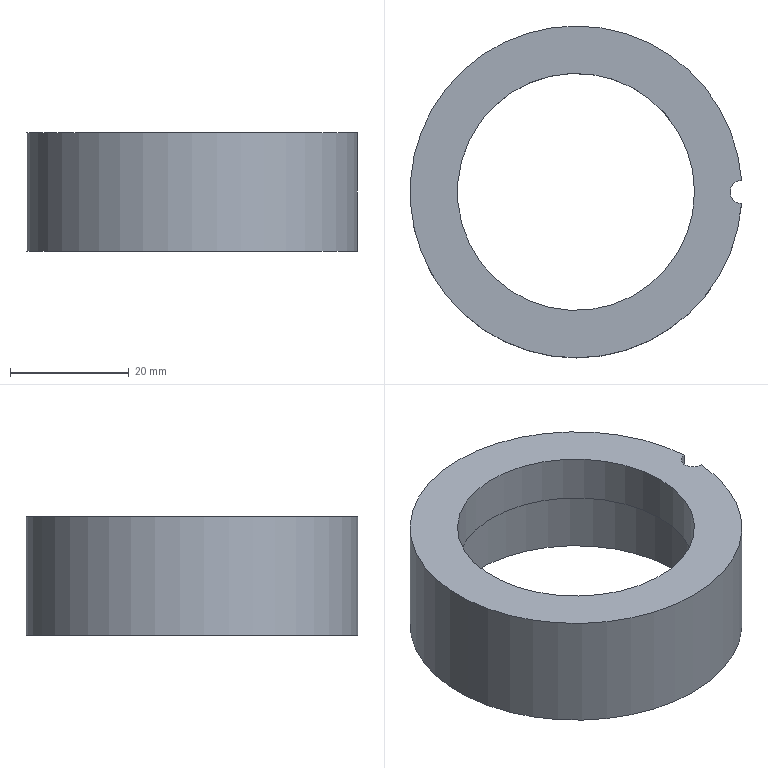Part | NX | features solid 2 | 1 solid | 7 faces | box 55.929 x 56 x 20 mm | volume 19140 mm3 | cylinder 4 | plane 3 | commonest cylinder face diameters 4 x1 40 x1 46 x1 56 x1
STEP:
#1=CARTESIAN_POINT('',(122.929,47.005,-50.));
#2=VERTEX_POINT('',#1);
#3=CARTESIAN_POINT('',(122.929,47.005,-30.));
#4=VERTEX_POINT('',#3);
#5=CARTESIAN_POINT('',(122.929,47.005,-40.));
#6=DIRECTION('',(0.,0.,1.));
#7=VECTOR('',#6,1000.);
#8=LINE('',#5,#7);
#9=EDGE_CURVE('',#2,#4,#8,.T.);
#10=ORIENTED_EDGE('',*,*,#9,.F.);
#11=CARTESIAN_POINT('',(122.929,43.008,-50.));
#12=VERTEX_POINT('',#11);
#13=CARTESIAN_POINT('',(95.,45.006,-50.));
#14=DIRECTION('',(0.,0.,1.));
#15=DIRECTION('',(1.,0.,0.));
#16=AXIS2_PLACEMENT_3D('',#13,#14,#15);
#17=CIRCLE('',#16,28.);
#18=EDGE_CURVE('',#2,#12,#17,.T.);
#19=ORIENTED_EDGE('',*,*,#18,.T.);
#20=CARTESIAN_POINT('',(122.929,43.008,-30.));
#21=VERTEX_POINT('',#20);
#22=CARTESIAN_POINT('',(122.929,43.008,-40.));
#23=DIRECTION('',(0.,0.,1.));
#24=VECTOR('',#23,1000.);
#25=LINE('',#22,#24);
#26=EDGE_CURVE('',#21,#12,#25,.F.);
#27=ORIENTED_EDGE('',*,*,#26,.F.);
#28=CARTESIAN_POINT('',(95.,45.006,-30.));
#29=DIRECTION('',(0.,0.,1.));
#30=DIRECTION('',(1.,0.,0.));
#31=AXIS2_PLACEMENT_3D('',#28,#29,#30);
#32=CIRCLE('',#31,28.);
#33=EDGE_CURVE('',#4,#21,#32,.T.);
#34=ORIENTED_EDGE('',*,*,#33,.F.);
#35=EDGE_LOOP('',(#10,#19,#27,#34));
#36=FACE_BOUND('',#35,.T.);
#37=CARTESIAN_POINT('',(95.,45.006,-50.));
#38=DIRECTION('',(0.,0.,1.));
#39=DIRECTION('',(1.,0.,0.));
#40=AXIS2_PLACEMENT_3D('',#37,#38,#39);
#41=CYLINDRICAL_SURFACE('',#40,28.);
#42=ADVANCED_FACE('',(#36),#41,.T.);
#43=CARTESIAN_POINT('',(118.,45.006,-50.));
#44=VERTEX_POINT('',#43);
#45=CARTESIAN_POINT('',(95.,45.006,-50.));
#46=DIRECTION('',(0.,0.,1.));
#47=DIRECTION('',(1.,0.,0.));
#48=AXIS2_PLACEMENT_3D('',#45,#46,#47);
#49=CIRCLE('',#48,23.);
#50=EDGE_CURVE('',#44,#44,#49,.T.);
#51=ORIENTED_EDGE('',*,*,#50,.T.);
#52=EDGE_LOOP('',(#51));
#53=FACE_BOUND('',#52,.T.);
#54=ORIENTED_EDGE('',*,*,#18,.F.);
#55=CARTESIAN_POINT('',(123.,45.006,-50.));
#56=DIRECTION('',(0.,0.,1.));
#57=DIRECTION('',(1.,0.,0.));
#58=AXIS2_PLACEMENT_3D('',#55,#56,#57);
#59=CIRCLE('',#58,2.);
#60=EDGE_CURVE('',#2,#12,#59,.T.);
#61=ORIENTED_EDGE('',*,*,#60,.T.);
#62=EDGE_LOOP('',(#54,#61));
#63=FACE_BOUND('',#62,.T.);
#64=CARTESIAN_POINT('',(95.,45.006,-50.));
#65=DIRECTION('',(0.,0.,1.));
#66=DIRECTION('',(1.,0.,0.));
#67=AXIS2_PLACEMENT_3D('',#64,#65,#66);
#68=PLANE('',#67);
#69=ADVANCED_FACE('',(#53,#63),#68,.F.);
#70=CARTESIAN_POINT('',(115.,45.006,-30.));
#71=VERTEX_POINT('',#70);
#72=CARTESIAN_POINT('',(95.,45.006,-30.));
#73=DIRECTION('',(0.,0.,1.));
#74=DIRECTION('',(1.,0.,0.));
#75=AXIS2_PLACEMENT_3D('',#72,#73,#74);
#76=CIRCLE('',#75,20.);
#77=EDGE_CURVE('',#71,#71,#76,.T.);
#78=ORIENTED_EDGE('',*,*,#77,.F.);
#79=EDGE_LOOP('',(#78));
#80=FACE_BOUND('',#79,.T.);
#81=CARTESIAN_POINT('',(123.,45.006,-30.));
#82=DIRECTION('',(0.,0.,1.));
#83=DIRECTION('',(1.,0.,0.));
#84=AXIS2_PLACEMENT_3D('',#81,#82,#83);
#85=CIRCLE('',#84,2.);
#86=EDGE_CURVE('',#4,#21,#85,.T.);
#87=ORIENTED_EDGE('',*,*,#86,.F.);
#88=ORIENTED_EDGE('',*,*,#33,.T.);
#89=EDGE_LOOP('',(#87,#88));
#90=FACE_BOUND('',#89,.T.);
#91=CARTESIAN_POINT('',(95.,45.006,-30.));
#92=DIRECTION('',(0.,0.,1.));
#93=DIRECTION('',(1.,0.,0.));
#94=AXIS2_PLACEMENT_3D('',#91,#92,#93);
#95=PLANE('',#94);
#96=ADVANCED_FACE('',(#80,#90),#95,.T.);
#97=ORIENTED_EDGE('',*,*,#50,.F.);
#98=EDGE_LOOP('',(#97));
#99=FACE_BOUND('',#98,.T.);
#100=CARTESIAN_POINT('',(118.,45.006,-38.));
#101=VERTEX_POINT('',#100);
#102=CARTESIAN_POINT('',(95.,45.006,-38.));
#103=DIRECTION('',(0.,0.,1.));
#104=DIRECTION('',(1.,0.,0.));
#105=AXIS2_PLACEMENT_3D('',#102,#103,#104);
#106=CIRCLE('',#105,23.);
#107=EDGE_CURVE('',#101,#101,#106,.T.);
#108=ORIENTED_EDGE('',*,*,#107,.T.);
#109=EDGE_LOOP('',(#108));
#110=FACE_BOUND('',#109,.T.);
#111=CARTESIAN_POINT('',(95.,45.006,-50.));
#112=DIRECTION('',(0.,0.,1.));
#113=DIRECTION('',(1.,0.,0.));
#114=AXIS2_PLACEMENT_3D('',#111,#112,#113);
#115=CYLINDRICAL_SURFACE('',#114,23.);
#116=ADVANCED_FACE('',(#99,#110),#115,.F.);
#117=CARTESIAN_POINT('',(115.,45.006,-38.));
#118=VERTEX_POINT('',#117);
#119=CARTESIAN_POINT('',(95.,45.006,-38.));
#120=DIRECTION('',(0.,0.,1.));
#121=DIRECTION('',(1.,0.,0.));
#122=AXIS2_PLACEMENT_3D('',#119,#120,#121);
#123=CIRCLE('',#122,20.);
#124=EDGE_CURVE('',#118,#118,#123,.T.);
#125=ORIENTED_EDGE('',*,*,#124,.T.);
#126=EDGE_LOOP('',(#125));
#127=FACE_BOUND('',#126,.T.);
#128=ORIENTED_EDGE('',*,*,#107,.F.);
#129=EDGE_LOOP('',(#128));
#130=FACE_BOUND('',#129,.T.);
#131=CARTESIAN_POINT('',(95.,45.006,-38.));
#132=DIRECTION('',(0.,0.,1.));
#133=DIRECTION('',(1.,0.,0.));
#134=AXIS2_PLACEMENT_3D('',#131,#132,#133);
#135=PLANE('',#134);
#136=ADVANCED_FACE('',(#127,#130),#135,.F.);
#137=ORIENTED_EDGE('',*,*,#9,.T.);
#138=ORIENTED_EDGE('',*,*,#86,.T.);
#139=ORIENTED_EDGE('',*,*,#26,.T.);
#140=ORIENTED_EDGE('',*,*,#60,.F.);
#141=EDGE_LOOP('',(#137,#138,#139,#140));
#142=FACE_BOUND('',#141,.T.);
#143=CARTESIAN_POINT('',(123.,45.006,-50.));
#144=DIRECTION('',(0.,0.,1.));
#145=DIRECTION('',(1.,0.,0.));
#146=AXIS2_PLACEMENT_3D('',#143,#144,#145);
#147=CYLINDRICAL_SURFACE('',#146,2.);
#148=ADVANCED_FACE('',(#142),#147,.F.);
#149=ORIENTED_EDGE('',*,*,#77,.T.);
#150=EDGE_LOOP('',(#149));
#151=FACE_BOUND('',#150,.T.);
#152=ORIENTED_EDGE('',*,*,#124,.F.);
#153=EDGE_LOOP('',(#152));
#154=FACE_BOUND('',#153,.T.);
#155=CARTESIAN_POINT('',(95.,45.006,-50.));
#156=DIRECTION('',(0.,0.,1.));
#157=DIRECTION('',(1.,0.,0.));
#158=AXIS2_PLACEMENT_3D('',#155,#156,#157);
#159=CYLINDRICAL_SURFACE('',#158,20.);
#160=ADVANCED_FACE('',(#151,#154),#159,.F.);
#161=CLOSED_SHELL('',(#42,#69,#96,#116,#136,#148,#160));
#162=MANIFOLD_SOLID_BREP('',#161);
#163=(LENGTH_UNIT()NAMED_UNIT(*)SI_UNIT(.MILLI.,.METRE.));
#164=UNCERTAINTY_MEASURE_WITH_UNIT(LENGTH_MEASURE(0.00001),#163,'','');
#165=(NAMED_UNIT(*)PLANE_ANGLE_UNIT()SI_UNIT($,.RADIAN.));
#166=(NAMED_UNIT(*)SI_UNIT($,.STERADIAN.)SOLID_ANGLE_UNIT());
#167=(GEOMETRIC_REPRESENTATION_CONTEXT(3)GLOBAL_UNCERTAINTY_ASSIGNED_CONTEXT((#164))GLOBAL_UNIT_ASSIGNED_CONTEXT((#163,#165,#166))REPRESENTATION_CONTEXT('',''));
#168=ADVANCED_BREP_SHAPE_REPRESENTATION('',(#162),#167);